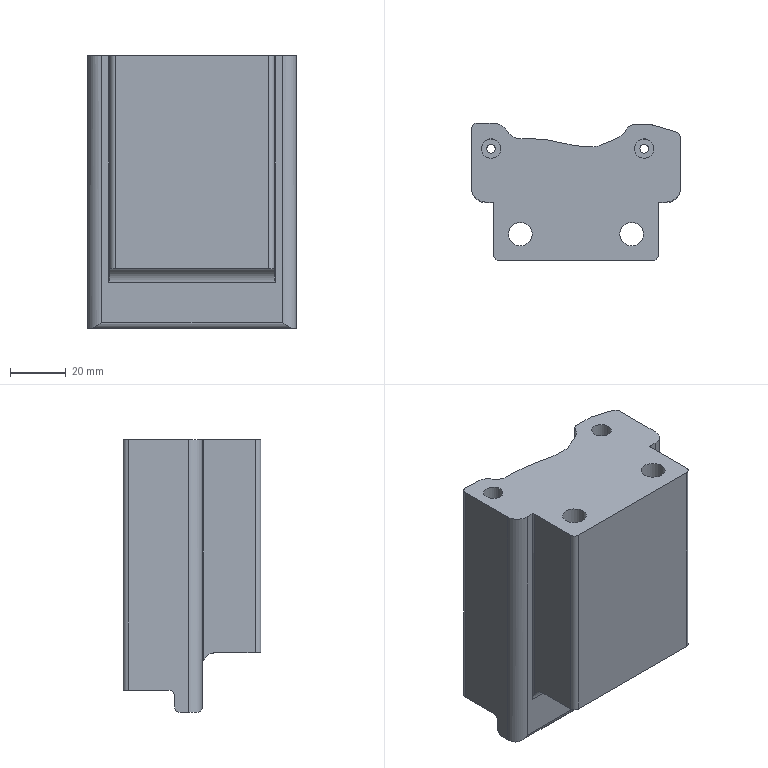Part | NX | features PU-6 2 | 1 solid | 48 faces | box 75 x 49.398 x 98 mm | volume 247595 mm3 | cylinder 22 | plane 19 | spline 7 | commonest cylinder face diameters 4 x9 10 x3 1 x2 3.101 x2 7 x2 8.506 x2